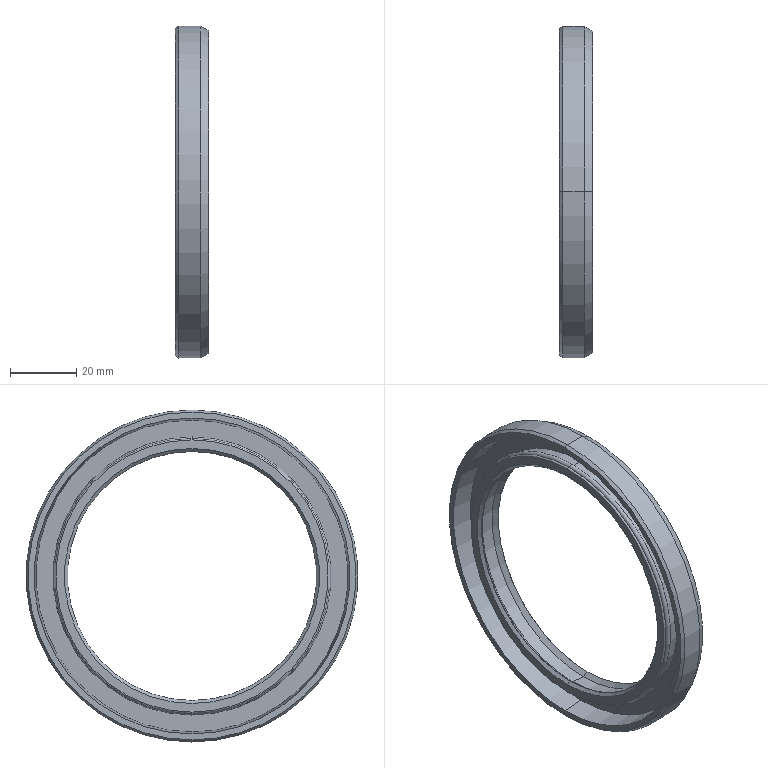Part | SolidWorks | features BaseBody 1 | 1 solid | 38 faces | box 10 x 100 x 100 mm | volume 19515 mm3 | cone 20 | torus 8 | cylinder 6 | plane 4 | commonest cylinder face diameters 78.465 x2 82.143 x2 100 x2
STEP:
#1=CARTESIAN_POINT('',(105.942,0.00006065,-37.5));
#2=VERTEX_POINT('',#1);
#3=CARTESIAN_POINT('',(105.871,0.0000607,-37.529));
#4=VERTEX_POINT('',#3);
#5=CARTESIAN_POINT('',(105.942,0.00006082,-37.6));
#6=DIRECTION('',(0.,-1.,-0.000001617));
#7=DIRECTION('',(0.,0.000001617,-1.));
#8=AXIS2_PLACEMENT_3D('',#5,#6,#7);
#9=CIRCLE('',#8,0.1);
#10=EDGE_CURVE('',#2,#4,#9,.T.);
#11=ORIENTED_EDGE('',*,*,#10,.F.);
#12=CARTESIAN_POINT('',(105.942,-0.00006065,37.5));
#13=VERTEX_POINT('',#12);
#14=CARTESIAN_POINT('',(105.942,0.,0.));
#15=DIRECTION('',(1.,0.,0.));
#16=DIRECTION('',(0.,1.,0.));
#17=AXIS2_PLACEMENT_3D('',#14,#15,#16);
#18=CIRCLE('',#17,37.5);
#19=EDGE_CURVE('',#2,#13,#18,.T.);
#20=ORIENTED_EDGE('',*,*,#19,.T.);
#21=CARTESIAN_POINT('',(105.871,-0.0000607,37.529));
#22=VERTEX_POINT('',#21);
#23=CARTESIAN_POINT('',(105.942,-0.00006082,37.6));
#24=DIRECTION('',(0.,1.,0.000001617));
#25=DIRECTION('',(0.,-0.000001617,1.));
#26=AXIS2_PLACEMENT_3D('',#23,#24,#25);
#27=CIRCLE('',#26,0.1);
#28=EDGE_CURVE('',#13,#22,#27,.T.);
#29=ORIENTED_EDGE('',*,*,#28,.T.);
#30=CARTESIAN_POINT('',(105.871,0.,37.529));
#31=VERTEX_POINT('',#30);
#32=CARTESIAN_POINT('',(105.871,0.,0.));
#33=DIRECTION('',(-1.,0.,0.));
#34=DIRECTION('',(0.,0.,-1.));
#35=AXIS2_PLACEMENT_3D('',#32,#33,#34);
#36=CIRCLE('',#35,37.529);
#37=EDGE_CURVE('',#22,#31,#36,.T.);
#38=ORIENTED_EDGE('',*,*,#37,.T.);
#39=CARTESIAN_POINT('',(105.871,0.,0.));
#40=DIRECTION('',(-1.,0.,0.));
#41=DIRECTION('',(0.,0.,-1.));
#42=AXIS2_PLACEMENT_3D('',#39,#40,#41);
#43=CIRCLE('',#42,37.529);
#44=EDGE_CURVE('',#31,#4,#43,.T.);
#45=ORIENTED_EDGE('',*,*,#44,.T.);
#46=EDGE_LOOP('',(#11,#20,#29,#38,#45));
#47=FACE_OUTER_BOUND('',#46,.T.);
#48=CARTESIAN_POINT('',(105.942,0.,0.));
#49=DIRECTION('',(1.,0.,0.));
#50=DIRECTION('',(0.,-0.000001617,1.));
#51=AXIS2_PLACEMENT_3D('',#48,#49,#50);
#52=TOROIDAL_SURFACE('',#51,37.6,0.1);
#53=ADVANCED_FACE('',(#47),#52,.T.);
#54=ORIENTED_EDGE('',*,*,#28,.F.);
#55=CARTESIAN_POINT('',(105.942,0.,0.));
#56=DIRECTION('',(1.,0.,0.));
#57=DIRECTION('',(0.,1.,0.));
#58=AXIS2_PLACEMENT_3D('',#55,#56,#57);
#59=CIRCLE('',#58,37.5);
#60=EDGE_CURVE('',#13,#2,#59,.T.);
#61=ORIENTED_EDGE('',*,*,#60,.T.);
#62=ORIENTED_EDGE('',*,*,#10,.T.);
#63=CARTESIAN_POINT('',(105.871,0.,-37.529));
#64=VERTEX_POINT('',#63);
#65=CARTESIAN_POINT('',(105.871,0.,0.));
#66=DIRECTION('',(-1.,0.,0.));
#67=DIRECTION('',(0.,0.,-1.));
#68=AXIS2_PLACEMENT_3D('',#65,#66,#67);
#69=CIRCLE('',#68,37.529);
#70=EDGE_CURVE('',#4,#64,#69,.T.);
#71=ORIENTED_EDGE('',*,*,#70,.T.);
#72=CARTESIAN_POINT('',(105.871,0.,0.));
#73=DIRECTION('',(-1.,0.,0.));
#74=DIRECTION('',(0.,0.,-1.));
#75=AXIS2_PLACEMENT_3D('',#72,#73,#74);
#76=CIRCLE('',#75,37.529);
#77=EDGE_CURVE('',#64,#22,#76,.T.);
#78=ORIENTED_EDGE('',*,*,#77,.T.);
#79=EDGE_LOOP('',(#54,#61,#62,#71,#78));
#80=FACE_OUTER_BOUND('',#79,.T.);
#81=CARTESIAN_POINT('',(105.942,0.,0.));
#82=DIRECTION('',(1.,0.,0.));
#83=DIRECTION('',(0.,-0.000001617,1.));
#84=AXIS2_PLACEMENT_3D('',#81,#82,#83);
#85=TOROIDAL_SURFACE('',#84,37.6,0.1);
#86=ADVANCED_FACE('',(#80),#85,.T.);
#87=ORIENTED_EDGE('',*,*,#60,.F.);
#88=CARTESIAN_POINT('',(106.002,-0.00006069,37.52));
#89=VERTEX_POINT('',#88);
#90=CARTESIAN_POINT('',(105.942,-0.00006082,37.6));
#91=DIRECTION('',(0.,1.,0.000001617));
#92=DIRECTION('',(0.,-0.000001617,1.));
#93=AXIS2_PLACEMENT_3D('',#90,#91,#92);
#94=CIRCLE('',#93,0.1);
#95=EDGE_CURVE('',#89,#13,#94,.T.);
#96=ORIENTED_EDGE('',*,*,#95,.F.);
#97=CARTESIAN_POINT('',(106.002,0.,-37.52));
#98=VERTEX_POINT('',#97);
#99=CARTESIAN_POINT('',(106.002,0.,0.));
#100=DIRECTION('',(-1.,0.,0.));
#101=DIRECTION('',(0.,0.,-1.));
#102=AXIS2_PLACEMENT_3D('',#99,#100,#101);
#103=CIRCLE('',#102,37.52);
#104=EDGE_CURVE('',#98,#89,#103,.T.);
#105=ORIENTED_EDGE('',*,*,#104,.F.);
#106=CARTESIAN_POINT('',(106.002,0.00006069,-37.52));
#107=VERTEX_POINT('',#106);
#108=CARTESIAN_POINT('',(106.002,0.,0.));
#109=DIRECTION('',(-1.,0.,0.));
#110=DIRECTION('',(0.,0.,-1.));
#111=AXIS2_PLACEMENT_3D('',#108,#109,#110);
#112=CIRCLE('',#111,37.52);
#113=EDGE_CURVE('',#107,#98,#112,.T.);
#114=ORIENTED_EDGE('',*,*,#113,.F.);
#115=CARTESIAN_POINT('',(105.942,0.00006082,-37.6));
#116=DIRECTION('',(0.,-1.,-0.000001617));
#117=DIRECTION('',(0.,0.000001617,-1.));
#118=AXIS2_PLACEMENT_3D('',#115,#116,#117);
#119=CIRCLE('',#118,0.1);
#120=EDGE_CURVE('',#107,#2,#119,.T.);
#121=ORIENTED_EDGE('',*,*,#120,.T.);
#122=EDGE_LOOP('',(#87,#96,#105,#114,#121));
#123=FACE_OUTER_BOUND('',#122,.T.);
#124=CARTESIAN_POINT('',(105.942,0.,0.));
#125=DIRECTION('',(1.,0.,0.));
#126=DIRECTION('',(0.,-0.000001617,1.));
#127=AXIS2_PLACEMENT_3D('',#124,#125,#126);
#128=TOROIDAL_SURFACE('',#127,37.6,0.1);
#129=ADVANCED_FACE('',(#123),#128,.T.);
#130=ORIENTED_EDGE('',*,*,#77,.F.);
#131=CARTESIAN_POINT('',(105.,0.,-38.4));
#132=VERTEX_POINT('',#131);
#133=CARTESIAN_POINT('',(142.4,0.,-1.));
#134=DIRECTION('',(-0.7071,0.,-0.7071));
#135=VECTOR('',#134,1000.);
#136=LINE('',#133,#135);
#137=EDGE_CURVE('',#64,#132,#136,.T.);
#138=ORIENTED_EDGE('',*,*,#137,.T.);
#139=CARTESIAN_POINT('',(105.,0.,38.4));
#140=VERTEX_POINT('',#139);
#141=CARTESIAN_POINT('',(105.,0.,0.));
#142=DIRECTION('',(-1.,0.,0.));
#143=DIRECTION('',(0.,0.,1.));
#144=AXIS2_PLACEMENT_3D('',#141,#142,#143);
#145=CIRCLE('',#144,38.4);
#146=EDGE_CURVE('',#132,#140,#145,.T.);
#147=ORIENTED_EDGE('',*,*,#146,.T.);
#148=CARTESIAN_POINT('',(142.4,0.,1.));
#149=DIRECTION('',(-0.7071,0.,0.7071));
#150=VECTOR('',#149,1000.);
#151=LINE('',#148,#150);
#152=EDGE_CURVE('',#31,#140,#151,.T.);
#153=ORIENTED_EDGE('',*,*,#152,.F.);
#154=ORIENTED_EDGE('',*,*,#37,.F.);
#155=EDGE_LOOP('',(#130,#138,#147,#153,#154));
#156=FACE_OUTER_BOUND('',#155,.T.);
#157=CARTESIAN_POINT('',(142.4,0.,0.));
#158=DIRECTION('',(-1.,0.,0.));
#159=DIRECTION('',(0.,0.,1.));
#160=AXIS2_PLACEMENT_3D('',#157,#158,#159);
#161=CONICAL_SURFACE('',#160,1.,0.7854);
#162=ADVANCED_FACE('',(#156),#161,.F.);
#163=CARTESIAN_POINT('',(105.,-0.000000008,40.996));
#164=VERTEX_POINT('',#163);
#165=CARTESIAN_POINT('',(105.,0.,-40.996));
#166=VERTEX_POINT('',#165);
#167=CARTESIAN_POINT('',(105.,0.,0.));
#168=DIRECTION('',(-1.,0.,0.));
#169=DIRECTION('',(0.,0.,-1.));
#170=AXIS2_PLACEMENT_3D('',#167,#168,#169);
#171=CIRCLE('',#170,40.996);
#172=EDGE_CURVE('',#164,#166,#171,.T.);
#173=ORIENTED_EDGE('',*,*,#172,.F.);
#174=CARTESIAN_POINT('',(105.799,0.,41.021));
#175=VERTEX_POINT('',#174);
#176=CARTESIAN_POINT('',(105.4,-0.000000007,40.996));
#177=DIRECTION('',(0.,1.,0.));
#178=DIRECTION('',(0.,0.,1.));
#179=AXIS2_PLACEMENT_3D('',#176,#177,#178);
#180=CIRCLE('',#179,0.4);
#181=EDGE_CURVE('',#164,#175,#180,.T.);
#182=ORIENTED_EDGE('',*,*,#181,.T.);
#183=CARTESIAN_POINT('',(105.799,0.000000027,-41.021));
#184=VERTEX_POINT('',#183);
#185=CARTESIAN_POINT('',(105.799,0.,0.));
#186=DIRECTION('',(-1.,0.,0.));
#187=DIRECTION('',(0.,0.,1.));
#188=AXIS2_PLACEMENT_3D('',#185,#186,#187);
#189=CIRCLE('',#188,41.021);
#190=EDGE_CURVE('',#175,#184,#189,.T.);
#191=ORIENTED_EDGE('',*,*,#190,.T.);
#192=CARTESIAN_POINT('',(105.4,0.000000007,-40.996));
#193=DIRECTION('',(0.,-1.,0.));
#194=DIRECTION('',(0.,0.,-1.));
#195=AXIS2_PLACEMENT_3D('',#192,#193,#194);
#196=CIRCLE('',#195,0.4);
#197=EDGE_CURVE('',#166,#184,#196,.T.);
#198=ORIENTED_EDGE('',*,*,#197,.F.);
#199=EDGE_LOOP('',(#173,#182,#191,#198));
#200=FACE_OUTER_BOUND('',#199,.T.);
#201=CARTESIAN_POINT('',(105.4,0.,0.));
#202=DIRECTION('',(1.,0.,0.));
#203=DIRECTION('',(0.,0.,-1.));
#204=AXIS2_PLACEMENT_3D('',#201,#202,#203);
#205=TOROIDAL_SURFACE('',#204,40.996,0.4);
#206=ADVANCED_FACE('',(#200),#205,.T.);
#207=CARTESIAN_POINT('',(105.799,0.,0.));
#208=DIRECTION('',(-1.,0.,0.));
#209=DIRECTION('',(0.,0.,1.));
#210=AXIS2_PLACEMENT_3D('',#207,#208,#209);
#211=CIRCLE('',#210,41.021);
#212=EDGE_CURVE('',#184,#175,#211,.T.);
#213=ORIENTED_EDGE('',*,*,#212,.F.);
#214=CARTESIAN_POINT('',(107.398,0.,-41.071));
#215=VERTEX_POINT('',#214);
#216=CARTESIAN_POINT('',(106.598,0.000000027,-41.071));
#217=DIRECTION('',(0.,-1.,-0.000000001));
#218=DIRECTION('',(0.,0.000000001,-1.));
#219=AXIS2_PLACEMENT_3D('',#216,#217,#218);
#220=CIRCLE('',#219,0.8);
#221=EDGE_CURVE('',#184,#215,#220,.T.);
#222=ORIENTED_EDGE('',*,*,#221,.T.);
#223=CARTESIAN_POINT('',(107.398,0.,41.071));
#224=VERTEX_POINT('',#223);
#225=CARTESIAN_POINT('',(107.398,0.,0.));
#226=DIRECTION('',(-1.,0.,0.));
#227=DIRECTION('',(0.,0.,-1.));
#228=AXIS2_PLACEMENT_3D('',#225,#226,#227);
#229=CIRCLE('',#228,41.071);
#230=EDGE_CURVE('',#215,#224,#229,.T.);
#231=ORIENTED_EDGE('',*,*,#230,.T.);
#232=CARTESIAN_POINT('',(106.598,-0.000000027,41.071));
#233=DIRECTION('',(0.,1.,0.000000001));
#234=DIRECTION('',(0.,-0.000000001,1.));
#235=AXIS2_PLACEMENT_3D('',#232,#233,#234);
#236=CIRCLE('',#235,0.8);
#237=EDGE_CURVE('',#175,#224,#236,.T.);
#238=ORIENTED_EDGE('',*,*,#237,.F.);
#239=EDGE_LOOP('',(#213,#222,#231,#238));
#240=FACE_OUTER_BOUND('',#239,.T.);
#241=CARTESIAN_POINT('',(106.598,0.,0.));
#242=DIRECTION('',(1.,0.,0.));
#243=DIRECTION('',(0.,-0.000000001,1.));
#244=AXIS2_PLACEMENT_3D('',#241,#242,#243);
#245=TOROIDAL_SURFACE('',#244,41.071,0.8);
#246=ADVANCED_FACE('',(#240),#245,.T.);
#247=CARTESIAN_POINT('',(107.398,0.,0.));
#248=DIRECTION('',(-1.,0.,0.));
#249=DIRECTION('',(0.,0.,-1.));
#250=AXIS2_PLACEMENT_3D('',#247,#248,#249);
#251=CIRCLE('',#250,41.071);
#252=EDGE_CURVE('',#224,#215,#251,.T.);
#253=ORIENTED_EDGE('',*,*,#252,.F.);
#254=CARTESIAN_POINT('',(110.667,0.,41.071));
#255=VERTEX_POINT('',#254);
#256=CARTESIAN_POINT('',(107.398,0.,41.071));
#257=DIRECTION('',(1.,0.,0.));
#258=VECTOR('',#257,1000.);
#259=LINE('',#256,#258);
#260=EDGE_CURVE('',#224,#255,#259,.T.);
#261=ORIENTED_EDGE('',*,*,#260,.T.);
#262=CARTESIAN_POINT('',(110.667,0.,-41.071));
#263=VERTEX_POINT('',#262);
#264=CARTESIAN_POINT('',(110.667,0.,0.));
#265=DIRECTION('',(-1.,0.,0.));
#266=DIRECTION('',(0.,0.,1.));
#267=AXIS2_PLACEMENT_3D('',#264,#265,#266);
#268=CIRCLE('',#267,41.071);
#269=EDGE_CURVE('',#255,#263,#268,.T.);
#270=ORIENTED_EDGE('',*,*,#269,.T.);
#271=CARTESIAN_POINT('',(107.398,0.,-41.071));
#272=DIRECTION('',(1.,0.,0.));
#273=VECTOR('',#272,1000.);
#274=LINE('',#271,#273);
#275=EDGE_CURVE('',#215,#263,#274,.T.);
#276=ORIENTED_EDGE('',*,*,#275,.F.);
#277=EDGE_LOOP('',(#253,#261,#270,#276));
#278=FACE_OUTER_BOUND('',#277,.T.);
#279=CARTESIAN_POINT('',(107.398,0.,0.));
#280=DIRECTION('',(1.,0.,0.));
#281=DIRECTION('',(0.,0.,-1.));
#282=AXIS2_PLACEMENT_3D('',#279,#280,#281);
#283=CYLINDRICAL_SURFACE('',#282,41.071);
#284=ADVANCED_FACE('',(#278),#283,.T.);
#285=CARTESIAN_POINT('',(110.667,0.,-46.982));
#286=VERTEX_POINT('',#285);
#287=CARTESIAN_POINT('',(110.667,0.,46.982));
#288=VERTEX_POINT('',#287);
#289=CARTESIAN_POINT('',(110.667,0.,0.));
#290=DIRECTION('',(-1.,0.,0.));
#291=DIRECTION('',(0.,0.,1.));
#292=AXIS2_PLACEMENT_3D('',#289,#290,#291);
#293=CIRCLE('',#292,46.982);
#294=EDGE_CURVE('',#286,#288,#293,.T.);
#295=ORIENTED_EDGE('',*,*,#294,.F.);
#296=CARTESIAN_POINT('',(104.,0.,-47.565));
#297=VERTEX_POINT('',#296);
#298=CARTESIAN_POINT('',(476.751,0.,-14.953));
#299=DIRECTION('',(-0.9962,0.,-0.08716));
#300=VECTOR('',#299,1000.);
#301=LINE('',#298,#300);
#302=EDGE_CURVE('',#286,#297,#301,.T.);
#303=ORIENTED_EDGE('',*,*,#302,.T.);
#304=CARTESIAN_POINT('',(104.,0.,47.565));
#305=VERTEX_POINT('',#304);
#306=CARTESIAN_POINT('',(104.,0.,0.));
#307=DIRECTION('',(-1.,0.,0.));
#308=DIRECTION('',(0.,0.,-1.));
#309=AXIS2_PLACEMENT_3D('',#306,#307,#308);
#310=CIRCLE('',#309,47.565);
#311=EDGE_CURVE('',#297,#305,#310,.T.);
#312=ORIENTED_EDGE('',*,*,#311,.T.);
#313=CARTESIAN_POINT('',(476.751,0.,14.953));
#314=DIRECTION('',(-0.9962,0.,0.08716));
#315=VECTOR('',#314,1000.);
#316=LINE('',#313,#315);
#317=EDGE_CURVE('',#288,#305,#316,.T.);
#318=ORIENTED_EDGE('',*,*,#317,.F.);
#319=EDGE_LOOP('',(#295,#303,#312,#318));
#320=FACE_OUTER_BOUND('',#319,.T.);
#321=CARTESIAN_POINT('',(476.751,0.,0.));
#322=DIRECTION('',(-1.,0.,0.));
#323=DIRECTION('',(0.,0.,1.));
#324=AXIS2_PLACEMENT_3D('',#321,#322,#323);
#325=CONICAL_SURFACE('',#324,14.953,0.08727);
#326=ADVANCED_FACE('',(#320),#325,.F.);
#327=CARTESIAN_POINT('',(104.,0.,49.351));
#328=VERTEX_POINT('',#327);
#329=CARTESIAN_POINT('',(104.,0.,-49.351));
#330=VERTEX_POINT('',#329);
#331=CARTESIAN_POINT('',(104.,0.,0.));
#332=DIRECTION('',(-1.,0.,0.));
#333=DIRECTION('',(0.,0.,-1.));
#334=AXIS2_PLACEMENT_3D('',#331,#332,#333);
#335=CIRCLE('',#334,49.351);
#336=EDGE_CURVE('',#328,#330,#335,.T.);
#337=ORIENTED_EDGE('',*,*,#336,.F.);
#338=CARTESIAN_POINT('',(105.,0.,50.));
#339=VERTEX_POINT('',#338);
#340=CARTESIAN_POINT('',(29.007,0.,0.6494));
#341=DIRECTION('',(0.8387,0.,0.5446));
#342=VECTOR('',#341,1000.);
#343=LINE('',#340,#342);
#344=EDGE_CURVE('',#328,#339,#343,.T.);
#345=ORIENTED_EDGE('',*,*,#344,.T.);
#346=CARTESIAN_POINT('',(105.,0.,-50.));
#347=VERTEX_POINT('',#346);
#348=CARTESIAN_POINT('',(105.,0.,0.));
#349=DIRECTION('',(-1.,0.,0.));
#350=DIRECTION('',(0.,0.,1.));
#351=AXIS2_PLACEMENT_3D('',#348,#349,#350);
#352=CIRCLE('',#351,50.);
#353=EDGE_CURVE('',#339,#347,#352,.T.);
#354=ORIENTED_EDGE('',*,*,#353,.T.);
#355=CARTESIAN_POINT('',(29.007,0.,-0.6494));
#356=DIRECTION('',(0.8387,0.,-0.5446));
#357=VECTOR('',#356,1000.);
#358=LINE('',#355,#357);
#359=EDGE_CURVE('',#330,#347,#358,.T.);
#360=ORIENTED_EDGE('',*,*,#359,.F.);
#361=EDGE_LOOP('',(#337,#345,#354,#360));
#362=FACE_OUTER_BOUND('',#361,.T.);
#363=CARTESIAN_POINT('',(29.007,0.,0.));
#364=DIRECTION('',(1.,0.,0.));
#365=DIRECTION('',(0.,0.,-1.));
#366=AXIS2_PLACEMENT_3D('',#363,#364,#365);
#367=CONICAL_SURFACE('',#366,0.6494,0.576);
#368=ADVANCED_FACE('',(#362),#367,.T.);
#369=CARTESIAN_POINT('',(105.,0.,0.));
#370=DIRECTION('',(-1.,0.,0.));
#371=DIRECTION('',(0.,0.,1.));
#372=AXIS2_PLACEMENT_3D('',#369,#370,#371);
#373=CIRCLE('',#372,50.);
#374=EDGE_CURVE('',#347,#339,#373,.T.);
#375=ORIENTED_EDGE('',*,*,#374,.F.);
#376=CARTESIAN_POINT('',(111.5,0.,-50.));
#377=VERTEX_POINT('',#376);
#378=CARTESIAN_POINT('',(105.,0.,-50.));
#379=DIRECTION('',(1.,0.,0.));
#380=VECTOR('',#379,1000.);
#381=LINE('',#378,#380);
#382=EDGE_CURVE('',#347,#377,#381,.T.);
#383=ORIENTED_EDGE('',*,*,#382,.T.);
#384=CARTESIAN_POINT('',(111.5,0.,50.));
#385=VERTEX_POINT('',#384);
#386=CARTESIAN_POINT('',(111.5,0.,0.));
#387=DIRECTION('',(-1.,0.,0.));
#388=DIRECTION('',(0.,0.,-1.));
#389=AXIS2_PLACEMENT_3D('',#386,#387,#388);
#390=CIRCLE('',#389,50.);
#391=EDGE_CURVE('',#377,#385,#390,.T.);
#392=ORIENTED_EDGE('',*,*,#391,.T.);
#393=CARTESIAN_POINT('',(105.,0.,50.));
#394=DIRECTION('',(1.,0.,0.));
#395=VECTOR('',#394,1000.);
#396=LINE('',#393,#395);
#397=EDGE_CURVE('',#339,#385,#396,.T.);
#398=ORIENTED_EDGE('',*,*,#397,.F.);
#399=EDGE_LOOP('',(#375,#383,#392,#398));
#400=FACE_OUTER_BOUND('',#399,.T.);
#401=CARTESIAN_POINT('',(105.,0.,0.));
#402=DIRECTION('',(1.,0.,0.));
#403=DIRECTION('',(0.,0.,1.));
#404=AXIS2_PLACEMENT_3D('',#401,#402,#403);
#405=CYLINDRICAL_SURFACE('',#404,50.);
#406=ADVANCED_FACE('',(#400),#405,.T.);
#407=CARTESIAN_POINT('',(114.,0.,48.557));
#408=VERTEX_POINT('',#407);
#409=CARTESIAN_POINT('',(114.,0.,-48.557));
#410=VERTEX_POINT('',#409);
#411=CARTESIAN_POINT('',(114.,0.,0.));
#412=DIRECTION('',(-1.,0.,0.));
#413=DIRECTION('',(0.,0.,1.));
#414=AXIS2_PLACEMENT_3D('',#411,#412,#413);
#415=CIRCLE('',#414,48.557);
#416=EDGE_CURVE('',#408,#410,#415,.T.);
#417=ORIENTED_EDGE('',*,*,#416,.T.);
#418=CARTESIAN_POINT('',(197.103,0.,-0.5774));
#419=DIRECTION('',(-0.866,0.,-0.5));
#420=VECTOR('',#419,1000.);
#421=LINE('',#418,#420);
#422=EDGE_CURVE('',#410,#377,#421,.T.);
#423=ORIENTED_EDGE('',*,*,#422,.T.);
#424=CARTESIAN_POINT('',(111.5,0.,0.));
#425=DIRECTION('',(-1.,0.,0.));
#426=DIRECTION('',(0.,0.,-1.));
#427=AXIS2_PLACEMENT_3D('',#424,#425,#426);
#428=CIRCLE('',#427,50.);
#429=EDGE_CURVE('',#385,#377,#428,.T.);
#430=ORIENTED_EDGE('',*,*,#429,.F.);
#431=CARTESIAN_POINT('',(197.103,0.,0.5774));
#432=DIRECTION('',(-0.866,0.,0.5));
#433=VECTOR('',#432,1000.);
#434=LINE('',#431,#433);
#435=EDGE_CURVE('',#408,#385,#434,.T.);
#436=ORIENTED_EDGE('',*,*,#435,.F.);
#437=EDGE_LOOP('',(#417,#423,#430,#436));
#438=FACE_OUTER_BOUND('',#437,.T.);
#439=CARTESIAN_POINT('',(197.103,0.,0.));
#440=DIRECTION('',(-1.,0.,0.));
#441=DIRECTION('',(0.,0.,1.));
#442=AXIS2_PLACEMENT_3D('',#439,#440,#441);
#443=CONICAL_SURFACE('',#442,0.5774,0.5236);
#444=ADVANCED_FACE('',(#438),#443,.T.);
#445=CARTESIAN_POINT('',(112.583,0.,39.232));
#446=VERTEX_POINT('',#445);
#447=CARTESIAN_POINT('',(112.583,0.,-39.232));
#448=VERTEX_POINT('',#447);
#449=CARTESIAN_POINT('',(112.583,0.,0.));
#450=DIRECTION('',(-1.,0.,0.));
#451=DIRECTION('',(0.,0.,1.));
#452=AXIS2_PLACEMENT_3D('',#449,#450,#451);
#453=CIRCLE('',#452,39.232);
#454=EDGE_CURVE('',#446,#448,#453,.T.);
#455=ORIENTED_EDGE('',*,*,#454,.T.);
#456=CARTESIAN_POINT('',(114.,0.,-39.232));
#457=VERTEX_POINT('',#456);
#458=CARTESIAN_POINT('',(112.583,0.,-39.232));
#459=DIRECTION('',(1.,0.,0.));
#460=VECTOR('',#459,1000.);
#461=LINE('',#458,#460);
#462=EDGE_CURVE('',#448,#457,#461,.T.);
#463=ORIENTED_EDGE('',*,*,#462,.T.);
#464=CARTESIAN_POINT('',(114.,0.,39.232));
#465=VERTEX_POINT('',#464);
#466=CARTESIAN_POINT('',(114.,0.,0.));
#467=DIRECTION('',(-1.,0.,0.));
#468=DIRECTION('',(0.,0.,-1.));
#469=AXIS2_PLACEMENT_3D('',#466,#467,#468);
#470=CIRCLE('',#469,39.232);
#471=EDGE_CURVE('',#465,#457,#470,.T.);
#472=ORIENTED_EDGE('',*,*,#471,.F.);
#473=CARTESIAN_POINT('',(112.583,0.,39.232));
#474=DIRECTION('',(1.,0.,0.));
#475=VECTOR('',#474,1000.);
#476=LINE('',#473,#475);
#477=EDGE_CURVE('',#446,#465,#476,.T.);
#478=ORIENTED_EDGE('',*,*,#477,.F.);
#479=EDGE_LOOP('',(#455,#463,#472,#478));
#480=FACE_OUTER_BOUND('',#479,.T.);
#481=CARTESIAN_POINT('',(112.583,0.,0.));
#482=DIRECTION('',(1.,0.,0.));
#483=DIRECTION('',(0.,0.,1.));
#484=AXIS2_PLACEMENT_3D('',#481,#482,#483);
#485=CYLINDRICAL_SURFACE('',#484,39.232);
#486=ADVANCED_FACE('',(#480),#485,.F.);
#487=CARTESIAN_POINT('',(113.714,0.,38.349));
#488=VERTEX_POINT('',#487);
#489=CARTESIAN_POINT('',(113.714,0.,-38.349));
#490=VERTEX_POINT('',#489);
#491=CARTESIAN_POINT('',(113.714,0.,0.));
#492=DIRECTION('',(-1.,0.,0.));
#493=DIRECTION('',(0.,0.,-1.));
#494=AXIS2_PLACEMENT_3D('',#491,#492,#493);
#495=CIRCLE('',#494,38.349);
#496=EDGE_CURVE('',#488,#490,#495,.T.);
#497=ORIENTED_EDGE('',*,*,#496,.T.);
#498=CARTESIAN_POINT('',(161.798,0.,-0.7813));
#499=DIRECTION('',(-0.788,0.,-0.6157));
#500=VECTOR('',#499,1000.);
#501=LINE('',#498,#500);
#502=EDGE_CURVE('',#490,#448,#501,.T.);
#503=ORIENTED_EDGE('',*,*,#502,.T.);
#504=ORIENTED_EDGE('',*,*,#454,.F.);
#505=CARTESIAN_POINT('',(161.798,0.,0.7813));
#506=DIRECTION('',(-0.788,0.,0.6157));
#507=VECTOR('',#506,1000.);
#508=LINE('',#505,#507);
#509=EDGE_CURVE('',#488,#446,#508,.T.);
#510=ORIENTED_EDGE('',*,*,#509,.F.);
#511=EDGE_LOOP('',(#497,#503,#504,#510));
#512=FACE_OUTER_BOUND('',#511,.T.);
#513=CARTESIAN_POINT('',(161.798,0.,0.));
#514=DIRECTION('',(-1.,0.,0.));
#515=DIRECTION('',(0.,0.,1.));
#516=AXIS2_PLACEMENT_3D('',#513,#514,#515);
#517=CONICAL_SURFACE('',#516,0.7813,0.6632);
#518=ADVANCED_FACE('',(#512),#517,.T.);
#519=CARTESIAN_POINT('',(113.275,0.,-37.786));
#520=VERTEX_POINT('',#519);
#521=CARTESIAN_POINT('',(113.275,0.,37.786));
#522=VERTEX_POINT('',#521);
#523=CARTESIAN_POINT('',(113.275,0.,0.));
#524=DIRECTION('',(-1.,0.,0.));
#525=DIRECTION('',(0.,0.,1.));
#526=AXIS2_PLACEMENT_3D('',#523,#524,#525);
#527=CIRCLE('',#526,37.786);
#528=EDGE_CURVE('',#520,#522,#527,.T.);
#529=ORIENTED_EDGE('',*,*,#528,.T.);
#530=CARTESIAN_POINT('',(84.753,0.,1.28));
#531=DIRECTION('',(0.6157,0.,0.788));
#532=VECTOR('',#531,1000.);
#533=LINE('',#530,#532);
#534=EDGE_CURVE('',#522,#488,#533,.T.);
#535=ORIENTED_EDGE('',*,*,#534,.T.);
#536=CARTESIAN_POINT('',(113.714,0.,0.));
#537=DIRECTION('',(-1.,0.,0.));
#538=DIRECTION('',(0.,0.,-1.));
#539=AXIS2_PLACEMENT_3D('',#536,#537,#538);
#540=CIRCLE('',#539,38.349);
#541=EDGE_CURVE('',#490,#488,#540,.T.);
#542=ORIENTED_EDGE('',*,*,#541,.F.);
#543=CARTESIAN_POINT('',(84.753,0.,-1.28));
#544=DIRECTION('',(0.6157,0.,-0.788));
#545=VECTOR('',#544,1000.);
#546=LINE('',#543,#545);
#547=EDGE_CURVE('',#520,#490,#546,.T.);
#548=ORIENTED_EDGE('',*,*,#547,.F.);
#549=EDGE_LOOP('',(#529,#535,#542,#548));
#550=FACE_OUTER_BOUND('',#549,.T.);
#551=CARTESIAN_POINT('',(84.753,0.,0.));
#552=DIRECTION('',(1.,0.,0.));
#553=DIRECTION('',(0.,0.,-1.));
#554=AXIS2_PLACEMENT_3D('',#551,#552,#553);
#555=CONICAL_SURFACE('',#554,1.28,0.9076);
#556=ADVANCED_FACE('',(#550),#555,.F.);
#557=ORIENTED_EDGE('',*,*,#528,.F.);
#558=CARTESIAN_POINT('',(111.773,0.,-38.959));
#559=VERTEX_POINT('',#558);
#560=CARTESIAN_POINT('',(160.638,0.,-0.7813));
#561=DIRECTION('',(-0.788,0.,-0.6157));
#562=VECTOR('',#561,1000.);
#563=LINE('',#560,#562);
#564=EDGE_CURVE('',#520,#559,#563,.T.);
#565=ORIENTED_EDGE('',*,*,#564,.T.);
#566=CARTESIAN_POINT('',(111.773,0.,38.959));
#567=VERTEX_POINT('',#566);
#568=CARTESIAN_POINT('',(111.773,0.,0.));
#569=DIRECTION('',(-1.,0.,0.));
#570=DIRECTION('',(0.,0.,-1.));
#571=AXIS2_PLACEMENT_3D('',#568,#569,#570);
#572=CIRCLE('',#571,38.959);
#573=EDGE_CURVE('',#559,#567,#572,.T.);
#574=ORIENTED_EDGE('',*,*,#573,.T.);
#575=CARTESIAN_POINT('',(160.638,0.,0.7813));
#576=DIRECTION('',(-0.788,0.,0.6157));
#577=VECTOR('',#576,1000.);
#578=LINE('',#575,#577);
#579=EDGE_CURVE('',#522,#567,#578,.T.);
#580=ORIENTED_EDGE('',*,*,#579,.F.);
#581=EDGE_LOOP('',(#557,#565,#574,#580));
#582=FACE_OUTER_BOUND('',#581,.T.);
#583=CARTESIAN_POINT('',(160.638,0.,0.));
#584=DIRECTION('',(-1.,0.,0.));
#585=DIRECTION('',(0.,0.,1.));
#586=AXIS2_PLACEMENT_3D('',#583,#584,#585);
#587=CONICAL_SURFACE('',#586,0.7813,0.6632);
#588=ADVANCED_FACE('',(#582),#587,.F.);
#589=CARTESIAN_POINT('',(106.977,0.,-38.37));
#590=VERTEX_POINT('',#589);
#591=CARTESIAN_POINT('',(106.977,0.,38.37));
#592=VERTEX_POINT('',#591);
#593=CARTESIAN_POINT('',(106.977,0.,0.));
#594=DIRECTION('',(-1.,0.,0.));
#595=DIRECTION('',(0.,0.,1.));
#596=AXIS2_PLACEMENT_3D('',#593,#594,#595);
#597=CIRCLE('',#596,38.37);
#598=EDGE_CURVE('',#590,#592,#597,.T.);
#599=ORIENTED_EDGE('',*,*,#598,.T.);
#600=CARTESIAN_POINT('',(-193.087,0.,1.527));
#601=DIRECTION('',(0.9925,0.,0.1219));
#602=VECTOR('',#601,1000.);
#603=LINE('',#600,#602);
#604=EDGE_CURVE('',#592,#567,#603,.T.);
#605=ORIENTED_EDGE('',*,*,#604,.T.);
#606=ORIENTED_EDGE('',*,*,#573,.F.);
#607=CARTESIAN_POINT('',(-193.087,0.,-1.527));
#608=DIRECTION('',(0.9925,0.,-0.1219));
#609=VECTOR('',#608,1000.);
#610=LINE('',#607,#609);
#611=EDGE_CURVE('',#590,#559,#610,.T.);
#612=ORIENTED_EDGE('',*,*,#611,.F.);
#613=EDGE_LOOP('',(#599,#605,#606,#612));
#614=FACE_OUTER_BOUND('',#613,.T.);
#615=CARTESIAN_POINT('',(-193.087,0.,0.));
#616=DIRECTION('',(1.,0.,0.));
#617=DIRECTION('',(0.,0.,-1.));
#618=AXIS2_PLACEMENT_3D('',#615,#616,#617);
#619=CONICAL_SURFACE('',#618,1.527,0.1222);
#620=ADVANCED_FACE('',(#614),#619,.F.);
#621=CARTESIAN_POINT('',(106.904,0.,-38.2));
#622=VERTEX_POINT('',#621);
#623=CARTESIAN_POINT('',(106.904,0.,38.2));
#624=VERTEX_POINT('',#623);
#625=CARTESIAN_POINT('',(106.904,0.,0.));
#626=DIRECTION('',(-1.,0.,0.));
#627=DIRECTION('',(0.,0.,-1.));
#628=AXIS2_PLACEMENT_3D('',#625,#626,#627);
#629=CIRCLE('',#628,38.2);
#630=EDGE_CURVE('',#622,#624,#629,.T.);
#631=ORIENTED_EDGE('',*,*,#630,.T.);
#632=CARTESIAN_POINT('',(91.689,0.,2.356));
#633=DIRECTION('',(0.3907,0.,0.9205));
#634=VECTOR('',#633,1000.);
#635=LINE('',#632,#634);
#636=EDGE_CURVE('',#624,#592,#635,.T.);
#637=ORIENTED_EDGE('',*,*,#636,.T.);
#638=ORIENTED_EDGE('',*,*,#598,.F.);
#639=CARTESIAN_POINT('',(91.689,0.,-2.356));
#640=DIRECTION('',(0.3907,0.,-0.9205));
#641=VECTOR('',#640,1000.);
#642=LINE('',#639,#641);
#643=EDGE_CURVE('',#622,#590,#642,.T.);
#644=ORIENTED_EDGE('',*,*,#643,.F.);
#645=EDGE_LOOP('',(#631,#637,#638,#644));
#646=FACE_OUTER_BOUND('',#645,.T.);
#647=CARTESIAN_POINT('',(91.689,0.,0.));
#648=DIRECTION('',(1.,0.,0.));
#649=DIRECTION('',(0.,0.,-1.));
#650=AXIS2_PLACEMENT_3D('',#647,#648,#649);
#651=CONICAL_SURFACE('',#650,2.356,1.169);
#652=ADVANCED_FACE('',(#646),#651,.F.);
#653=ORIENTED_EDGE('',*,*,#104,.T.);
#654=CARTESIAN_POINT('',(106.002,0.,37.52));
#655=VERTEX_POINT('',#654);
#656=CARTESIAN_POINT('',(106.002,0.,0.));
#657=DIRECTION('',(-1.,0.,0.));
#658=DIRECTION('',(0.,0.,-1.));
#659=AXIS2_PLACEMENT_3D('',#656,#657,#658);
#660=CIRCLE('',#659,37.52);
#661=EDGE_CURVE('',#89,#655,#660,.T.);
#662=ORIENTED_EDGE('',*,*,#661,.T.);
#663=CARTESIAN_POINT('',(57.211,0.,0.7536));
#664=DIRECTION('',(0.7986,0.,0.6018));
#665=VECTOR('',#664,1000.);
#666=LINE('',#663,#665);
#667=EDGE_CURVE('',#655,#624,#666,.T.);
#668=ORIENTED_EDGE('',*,*,#667,.T.);
#669=ORIENTED_EDGE('',*,*,#630,.F.);
#670=CARTESIAN_POINT('',(57.211,0.,-0.7536));
#671=DIRECTION('',(0.7986,0.,-0.6018));
#672=VECTOR('',#671,1000.);
#673=LINE('',#670,#672);
#674=EDGE_CURVE('',#98,#622,#673,.T.);
#675=ORIENTED_EDGE('',*,*,#674,.F.);
#676=EDGE_LOOP('',(#653,#662,#668,#669,#675));
#677=FACE_OUTER_BOUND('',#676,.T.);
#678=CARTESIAN_POINT('',(57.211,0.,0.));
#679=DIRECTION('',(1.,0.,0.));
#680=DIRECTION('',(0.,0.,-1.));
#681=AXIS2_PLACEMENT_3D('',#678,#679,#680);
#682=CONICAL_SURFACE('',#681,0.7536,0.6458);
#683=ADVANCED_FACE('',(#677),#682,.F.);
#684=ORIENTED_EDGE('',*,*,#667,.F.);
#685=CARTESIAN_POINT('',(106.002,0.,0.));
#686=DIRECTION('',(-1.,0.,0.));
#687=DIRECTION('',(0.,0.,-1.));
#688=AXIS2_PLACEMENT_3D('',#685,#686,#687);
#689=CIRCLE('',#688,37.52);
#690=EDGE_CURVE('',#655,#107,#689,.T.);
#691=ORIENTED_EDGE('',*,*,#690,.T.);
#692=ORIENTED_EDGE('',*,*,#113,.T.);
#693=ORIENTED_EDGE('',*,*,#674,.T.);
#694=CARTESIAN_POINT('',(106.904,0.,0.));
#695=DIRECTION('',(-1.,0.,0.));
#696=DIRECTION('',(0.,0.,-1.));
#697=AXIS2_PLACEMENT_3D('',#694,#695,#696);
#698=CIRCLE('',#697,38.2);
#699=EDGE_CURVE('',#624,#622,#698,.T.);
#700=ORIENTED_EDGE('',*,*,#699,.F.);
#701=EDGE_LOOP('',(#684,#691,#692,#693,#700));
#702=FACE_OUTER_BOUND('',#701,.T.);
#703=CARTESIAN_POINT('',(57.211,0.,0.));
#704=DIRECTION('',(1.,0.,0.));
#705=DIRECTION('',(0.,0.,-1.));
#706=AXIS2_PLACEMENT_3D('',#703,#704,#705);
#707=CONICAL_SURFACE('',#706,0.7536,0.6458);
#708=ADVANCED_FACE('',(#702),#707,.F.);
#709=ORIENTED_EDGE('',*,*,#636,.F.);
#710=ORIENTED_EDGE('',*,*,#699,.T.);
#711=ORIENTED_EDGE('',*,*,#643,.T.);
#712=CARTESIAN_POINT('',(106.977,0.,0.));
#713=DIRECTION('',(-1.,0.,0.));
#714=DIRECTION('',(0.,0.,1.));
#715=AXIS2_PLACEMENT_3D('',#712,#713,#714);
#716=CIRCLE('',#715,38.37);
#717=EDGE_CURVE('',#592,#590,#716,.T.);
#718=ORIENTED_EDGE('',*,*,#717,.F.);
#719=EDGE_LOOP('',(#709,#710,#711,#718));
#720=FACE_OUTER_BOUND('',#719,.T.);
#721=CARTESIAN_POINT('',(91.689,0.,0.));
#722=DIRECTION('',(1.,0.,0.));
#723=DIRECTION('',(0.,0.,-1.));
#724=AXIS2_PLACEMENT_3D('',#721,#722,#723);
#725=CONICAL_SURFACE('',#724,2.356,1.169);
#726=ADVANCED_FACE('',(#720),#725,.F.);
#727=ORIENTED_EDGE('',*,*,#604,.F.);
#728=ORIENTED_EDGE('',*,*,#717,.T.);
#729=ORIENTED_EDGE('',*,*,#611,.T.);
#730=CARTESIAN_POINT('',(111.773,0.,0.));
#731=DIRECTION('',(-1.,0.,0.));
#732=DIRECTION('',(0.,0.,-1.));
#733=AXIS2_PLACEMENT_3D('',#730,#731,#732);
#734=CIRCLE('',#733,38.959);
#735=EDGE_CURVE('',#567,#559,#734,.T.);
#736=ORIENTED_EDGE('',*,*,#735,.F.);
#737=EDGE_LOOP('',(#727,#728,#729,#736));
#738=FACE_OUTER_BOUND('',#737,.T.);
#739=CARTESIAN_POINT('',(-193.087,0.,0.));
#740=DIRECTION('',(1.,0.,0.));
#741=DIRECTION('',(0.,0.,-1.));
#742=AXIS2_PLACEMENT_3D('',#739,#740,#741);
#743=CONICAL_SURFACE('',#742,1.527,0.1222);
#744=ADVANCED_FACE('',(#738),#743,.F.);
#745=ORIENTED_EDGE('',*,*,#564,.F.);
#746=CARTESIAN_POINT('',(113.275,0.,0.));
#747=DIRECTION('',(-1.,0.,0.));
#748=DIRECTION('',(0.,0.,1.));
#749=AXIS2_PLACEMENT_3D('',#746,#747,#748);
#750=CIRCLE('',#749,37.786);
#751=EDGE_CURVE('',#522,#520,#750,.T.);
#752=ORIENTED_EDGE('',*,*,#751,.F.);
#753=ORIENTED_EDGE('',*,*,#579,.T.);
#754=ORIENTED_EDGE('',*,*,#735,.T.);
#755=EDGE_LOOP('',(#745,#752,#753,#754));
#756=FACE_OUTER_BOUND('',#755,.T.);
#757=CARTESIAN_POINT('',(160.638,0.,0.));
#758=DIRECTION('',(-1.,0.,0.));
#759=DIRECTION('',(0.,0.,1.));
#760=AXIS2_PLACEMENT_3D('',#757,#758,#759);
#761=CONICAL_SURFACE('',#760,0.7813,0.6632);
#762=ADVANCED_FACE('',(#756),#761,.F.);
#763=ORIENTED_EDGE('',*,*,#534,.F.);
#764=ORIENTED_EDGE('',*,*,#751,.T.);
#765=ORIENTED_EDGE('',*,*,#547,.T.);
#766=ORIENTED_EDGE('',*,*,#496,.F.);
#767=EDGE_LOOP('',(#763,#764,#765,#766));
#768=FACE_OUTER_BOUND('',#767,.T.);
#769=CARTESIAN_POINT('',(84.753,0.,0.));
#770=DIRECTION('',(1.,0.,0.));
#771=DIRECTION('',(0.,0.,-1.));
#772=AXIS2_PLACEMENT_3D('',#769,#770,#771);
#773=CONICAL_SURFACE('',#772,1.28,0.9076);
#774=ADVANCED_FACE('',(#768),#773,.F.);
#775=ORIENTED_EDGE('',*,*,#502,.F.);
#776=ORIENTED_EDGE('',*,*,#541,.T.);
#777=ORIENTED_EDGE('',*,*,#509,.T.);
#778=CARTESIAN_POINT('',(112.583,0.,0.));
#779=DIRECTION('',(-1.,0.,0.));
#780=DIRECTION('',(0.,0.,1.));
#781=AXIS2_PLACEMENT_3D('',#778,#779,#780);
#782=CIRCLE('',#781,39.232);
#783=EDGE_CURVE('',#448,#446,#782,.T.);
#784=ORIENTED_EDGE('',*,*,#783,.F.);
#785=EDGE_LOOP('',(#775,#776,#777,#784));
#786=FACE_OUTER_BOUND('',#785,.T.);
#787=CARTESIAN_POINT('',(161.798,0.,0.));
#788=DIRECTION('',(-1.,0.,0.));
#789=DIRECTION('',(0.,0.,1.));
#790=AXIS2_PLACEMENT_3D('',#787,#788,#789);
#791=CONICAL_SURFACE('',#790,0.7813,0.6632);
#792=ADVANCED_FACE('',(#786),#791,.T.);
#793=ORIENTED_EDGE('',*,*,#462,.F.);
#794=ORIENTED_EDGE('',*,*,#783,.T.);
#795=ORIENTED_EDGE('',*,*,#477,.T.);
#796=CARTESIAN_POINT('',(114.,0.,0.));
#797=DIRECTION('',(-1.,0.,0.));
#798=DIRECTION('',(0.,0.,-1.));
#799=AXIS2_PLACEMENT_3D('',#796,#797,#798);
#800=CIRCLE('',#799,39.232);
#801=EDGE_CURVE('',#457,#465,#800,.T.);
#802=ORIENTED_EDGE('',*,*,#801,.F.);
#803=EDGE_LOOP('',(#793,#794,#795,#802));
#804=FACE_OUTER_BOUND('',#803,.T.);
#805=CARTESIAN_POINT('',(112.583,0.,0.));
#806=DIRECTION('',(1.,0.,0.));
#807=DIRECTION('',(0.,0.,1.));
#808=AXIS2_PLACEMENT_3D('',#805,#806,#807);
#809=CYLINDRICAL_SURFACE('',#808,39.232);
#810=ADVANCED_FACE('',(#804),#809,.F.);
#811=ORIENTED_EDGE('',*,*,#471,.T.);
#812=ORIENTED_EDGE('',*,*,#801,.T.);
#813=EDGE_LOOP('',(#811,#812));
#814=FACE_BOUND('',#813,.T.);
#815=ORIENTED_EDGE('',*,*,#416,.F.);
#816=CARTESIAN_POINT('',(114.,0.,0.));
#817=DIRECTION('',(-1.,0.,0.));
#818=DIRECTION('',(0.,0.,1.));
#819=AXIS2_PLACEMENT_3D('',#816,#817,#818);
#820=CIRCLE('',#819,48.557);
#821=EDGE_CURVE('',#410,#408,#820,.T.);
#822=ORIENTED_EDGE('',*,*,#821,.F.);
#823=EDGE_LOOP('',(#815,#822));
#824=FACE_OUTER_BOUND('',#823,.T.);
#825=CARTESIAN_POINT('',(114.,48.557,0.));
#826=DIRECTION('',(1.,0.,0.));
#827=DIRECTION('',(0.,-1.,0.));
#828=AXIS2_PLACEMENT_3D('',#825,#826,#827);
#829=PLANE('',#828);
#830=ADVANCED_FACE('',(#814,#824),#829,.T.);
#831=ORIENTED_EDGE('',*,*,#422,.F.);
#832=ORIENTED_EDGE('',*,*,#821,.T.);
#833=ORIENTED_EDGE('',*,*,#435,.T.);
#834=ORIENTED_EDGE('',*,*,#391,.F.);
#835=EDGE_LOOP('',(#831,#832,#833,#834));
#836=FACE_OUTER_BOUND('',#835,.T.);
#837=CARTESIAN_POINT('',(197.103,0.,0.));
#838=DIRECTION('',(-1.,0.,0.));
#839=DIRECTION('',(0.,0.,1.));
#840=AXIS2_PLACEMENT_3D('',#837,#838,#839);
#841=CONICAL_SURFACE('',#840,0.5774,0.5236);
#842=ADVANCED_FACE('',(#836),#841,.T.);
#843=ORIENTED_EDGE('',*,*,#382,.F.);
#844=ORIENTED_EDGE('',*,*,#353,.F.);
#845=ORIENTED_EDGE('',*,*,#397,.T.);
#846=ORIENTED_EDGE('',*,*,#429,.T.);
#847=EDGE_LOOP('',(#843,#844,#845,#846));
#848=FACE_OUTER_BOUND('',#847,.T.);
#849=CARTESIAN_POINT('',(105.,0.,0.));
#850=DIRECTION('',(1.,0.,0.));
#851=DIRECTION('',(0.,0.,1.));
#852=AXIS2_PLACEMENT_3D('',#849,#850,#851);
#853=CYLINDRICAL_SURFACE('',#852,50.);
#854=ADVANCED_FACE('',(#848),#853,.T.);
#855=ORIENTED_EDGE('',*,*,#344,.F.);
#856=CARTESIAN_POINT('',(104.,0.,0.));
#857=DIRECTION('',(-1.,0.,0.));
#858=DIRECTION('',(0.,0.,-1.));
#859=AXIS2_PLACEMENT_3D('',#856,#857,#858);
#860=CIRCLE('',#859,49.351);
#861=EDGE_CURVE('',#330,#328,#860,.T.);
#862=ORIENTED_EDGE('',*,*,#861,.F.);
#863=ORIENTED_EDGE('',*,*,#359,.T.);
#864=ORIENTED_EDGE('',*,*,#374,.T.);
#865=EDGE_LOOP('',(#855,#862,#863,#864));
#866=FACE_OUTER_BOUND('',#865,.T.);
#867=CARTESIAN_POINT('',(29.007,0.,0.));
#868=DIRECTION('',(1.,0.,0.));
#869=DIRECTION('',(0.,0.,-1.));
#870=AXIS2_PLACEMENT_3D('',#867,#868,#869);
#871=CONICAL_SURFACE('',#870,0.6494,0.576);
#872=ADVANCED_FACE('',(#866),#871,.T.);
#873=CARTESIAN_POINT('',(104.,0.,0.));
#874=DIRECTION('',(-1.,0.,0.));
#875=DIRECTION('',(0.,0.,-1.));
#876=AXIS2_PLACEMENT_3D('',#873,#874,#875);
#877=CIRCLE('',#876,47.565);
#878=EDGE_CURVE('',#305,#297,#877,.T.);
#879=ORIENTED_EDGE('',*,*,#878,.F.);
#880=ORIENTED_EDGE('',*,*,#311,.F.);
#881=EDGE_LOOP('',(#879,#880));
#882=FACE_BOUND('',#881,.T.);
#883=ORIENTED_EDGE('',*,*,#861,.T.);
#884=ORIENTED_EDGE('',*,*,#336,.T.);
#885=EDGE_LOOP('',(#883,#884));
#886=FACE_OUTER_BOUND('',#885,.T.);
#887=CARTESIAN_POINT('',(104.,47.565,0.));
#888=DIRECTION('',(-1.,0.,0.));
#889=DIRECTION('',(0.,0.,1.));
#890=AXIS2_PLACEMENT_3D('',#887,#888,#889);
#891=PLANE('',#890);
#892=ADVANCED_FACE('',(#882,#886),#891,.T.);
#893=ORIENTED_EDGE('',*,*,#302,.F.);
#894=CARTESIAN_POINT('',(110.667,0.,0.));
#895=DIRECTION('',(-1.,0.,0.));
#896=DIRECTION('',(0.,0.,1.));
#897=AXIS2_PLACEMENT_3D('',#894,#895,#896);
#898=CIRCLE('',#897,46.982);
#899=EDGE_CURVE('',#288,#286,#898,.T.);
#900=ORIENTED_EDGE('',*,*,#899,.F.);
#901=ORIENTED_EDGE('',*,*,#317,.T.);
#902=ORIENTED_EDGE('',*,*,#878,.T.);
#903=EDGE_LOOP('',(#893,#900,#901,#902));
#904=FACE_OUTER_BOUND('',#903,.T.);
#905=CARTESIAN_POINT('',(476.751,0.,0.));
#906=DIRECTION('',(-1.,0.,0.));
#907=DIRECTION('',(0.,0.,1.));
#908=AXIS2_PLACEMENT_3D('',#905,#906,#907);
#909=CONICAL_SURFACE('',#908,14.953,0.08727);
#910=ADVANCED_FACE('',(#904),#909,.F.);
#911=CARTESIAN_POINT('',(110.667,0.,0.));
#912=DIRECTION('',(-1.,0.,0.));
#913=DIRECTION('',(0.,0.,1.));
#914=AXIS2_PLACEMENT_3D('',#911,#912,#913);
#915=CIRCLE('',#914,41.071);
#916=EDGE_CURVE('',#263,#255,#915,.T.);
#917=ORIENTED_EDGE('',*,*,#916,.F.);
#918=ORIENTED_EDGE('',*,*,#269,.F.);
#919=EDGE_LOOP('',(#917,#918));
#920=FACE_BOUND('',#919,.T.);
#921=ORIENTED_EDGE('',*,*,#899,.T.);
#922=ORIENTED_EDGE('',*,*,#294,.T.);
#923=EDGE_LOOP('',(#921,#922));
#924=FACE_OUTER_BOUND('',#923,.T.);
#925=CARTESIAN_POINT('',(110.667,41.071,0.));
#926=DIRECTION('',(-1.,0.,0.));
#927=DIRECTION('',(0.,0.,1.));
#928=AXIS2_PLACEMENT_3D('',#925,#926,#927);
#929=PLANE('',#928);
#930=ADVANCED_FACE('',(#920,#924),#929,.T.);
#931=ORIENTED_EDGE('',*,*,#260,.F.);
#932=ORIENTED_EDGE('',*,*,#230,.F.);
#933=ORIENTED_EDGE('',*,*,#275,.T.);
#934=ORIENTED_EDGE('',*,*,#916,.T.);
#935=EDGE_LOOP('',(#931,#932,#933,#934));
#936=FACE_OUTER_BOUND('',#935,.T.);
#937=CARTESIAN_POINT('',(107.398,0.,0.));
#938=DIRECTION('',(1.,0.,0.));
#939=DIRECTION('',(0.,0.,-1.));
#940=AXIS2_PLACEMENT_3D('',#937,#938,#939);
#941=CYLINDRICAL_SURFACE('',#940,41.071);
#942=ADVANCED_FACE('',(#936),#941,.T.);
#943=ORIENTED_EDGE('',*,*,#221,.F.);
#944=ORIENTED_EDGE('',*,*,#190,.F.);
#945=ORIENTED_EDGE('',*,*,#237,.T.);
#946=ORIENTED_EDGE('',*,*,#252,.T.);
#947=EDGE_LOOP('',(#943,#944,#945,#946));
#948=FACE_OUTER_BOUND('',#947,.T.);
#949=CARTESIAN_POINT('',(106.598,0.,0.));
#950=DIRECTION('',(1.,0.,0.));
#951=DIRECTION('',(0.,-0.000000001,1.));
#952=AXIS2_PLACEMENT_3D('',#949,#950,#951);
#953=TOROIDAL_SURFACE('',#952,41.071,0.8);
#954=ADVANCED_FACE('',(#948),#953,.T.);
#955=ORIENTED_EDGE('',*,*,#181,.F.);
#956=CARTESIAN_POINT('',(105.,0.,0.));
#957=DIRECTION('',(-1.,0.,0.));
#958=DIRECTION('',(0.,0.,-1.));
#959=AXIS2_PLACEMENT_3D('',#956,#957,#958);
#960=CIRCLE('',#959,40.996);
#961=EDGE_CURVE('',#166,#164,#960,.T.);
#962=ORIENTED_EDGE('',*,*,#961,.F.);
#963=ORIENTED_EDGE('',*,*,#197,.T.);
#964=ORIENTED_EDGE('',*,*,#212,.T.);
#965=EDGE_LOOP('',(#955,#962,#963,#964));
#966=FACE_OUTER_BOUND('',#965,.T.);
#967=CARTESIAN_POINT('',(105.4,0.,0.));
#968=DIRECTION('',(1.,0.,0.));
#969=DIRECTION('',(0.,0.,-1.));
#970=AXIS2_PLACEMENT_3D('',#967,#968,#969);
#971=TOROIDAL_SURFACE('',#970,40.996,0.4);
#972=ADVANCED_FACE('',(#966),#971,.T.);
#973=CARTESIAN_POINT('',(105.,0.,0.));
#974=DIRECTION('',(-1.,0.,0.));
#975=DIRECTION('',(0.,0.,1.));
#976=AXIS2_PLACEMENT_3D('',#973,#974,#975);
#977=CIRCLE('',#976,38.4);
#978=EDGE_CURVE('',#140,#132,#977,.T.);
#979=ORIENTED_EDGE('',*,*,#978,.F.);
#980=ORIENTED_EDGE('',*,*,#146,.F.);
#981=EDGE_LOOP('',(#979,#980));
#982=FACE_BOUND('',#981,.T.);
#983=ORIENTED_EDGE('',*,*,#961,.T.);
#984=ORIENTED_EDGE('',*,*,#172,.T.);
#985=EDGE_LOOP('',(#983,#984));
#986=FACE_OUTER_BOUND('',#985,.T.);
#987=CARTESIAN_POINT('',(105.,38.4,0.));
#988=DIRECTION('',(-1.,0.,0.));
#989=DIRECTION('',(0.,0.,1.));
#990=AXIS2_PLACEMENT_3D('',#987,#988,#989);
#991=PLANE('',#990);
#992=ADVANCED_FACE('',(#982,#986),#991,.T.);
#993=ORIENTED_EDGE('',*,*,#137,.F.);
#994=ORIENTED_EDGE('',*,*,#70,.F.);
#995=ORIENTED_EDGE('',*,*,#44,.F.);
#996=ORIENTED_EDGE('',*,*,#152,.T.);
#997=ORIENTED_EDGE('',*,*,#978,.T.);
#998=EDGE_LOOP('',(#993,#994,#995,#996,#997));
#999=FACE_OUTER_BOUND('',#998,.T.);
#1000=CARTESIAN_POINT('',(142.4,0.,0.));
#1001=DIRECTION('',(-1.,0.,0.));
#1002=DIRECTION('',(0.,0.,1.));
#1003=AXIS2_PLACEMENT_3D('',#1000,#1001,#1002);
#1004=CONICAL_SURFACE('',#1003,1.,0.7854);
#1005=ADVANCED_FACE('',(#999),#1004,.F.);
#1006=ORIENTED_EDGE('',*,*,#19,.F.);
#1007=ORIENTED_EDGE('',*,*,#120,.F.);
#1008=ORIENTED_EDGE('',*,*,#690,.F.);
#1009=ORIENTED_EDGE('',*,*,#661,.F.);
#1010=ORIENTED_EDGE('',*,*,#95,.T.);
#1011=EDGE_LOOP('',(#1006,#1007,#1008,#1009,#1010));
#1012=FACE_OUTER_BOUND('',#1011,.T.);
#1013=CARTESIAN_POINT('',(105.942,0.,0.));
#1014=DIRECTION('',(1.,0.,0.));
#1015=DIRECTION('',(0.,-0.000001617,1.));
#1016=AXIS2_PLACEMENT_3D('',#1013,#1014,#1015);
#1017=TOROIDAL_SURFACE('',#1016,37.6,0.1);
#1018=ADVANCED_FACE('',(#1012),#1017,.T.);
#1019=CLOSED_SHELL('',(#53,#86,#129,#162,#206,#246,#284,#326,#368,#406,#444,#486,#518,#556,#588,#620,#652,#683,#708,#726,#744,#762,#774,#792,#810,#830,#842,#854,#872,#892,#910,#930,#942,#954,#972,#992,#1005,#1018));
#1020=MANIFOLD_SOLID_BREP('',#1019);
#1021=CARTESIAN_POINT('',(0.,0.,0.));
#1022=DIRECTION('',(0.,0.,1.));
#1023=DIRECTION('',(1.,0.,0.));
#1024=AXIS2_PLACEMENT_3D('',#1021,#1022,#1023);
#1025=(LENGTH_UNIT()NAMED_UNIT(*)SI_UNIT(.MILLI.,.METRE.));
#1026=UNCERTAINTY_MEASURE_WITH_UNIT(LENGTH_MEASURE(0.00001),#1025,'','');
#1027=(NAMED_UNIT(*)PLANE_ANGLE_UNIT()SI_UNIT($,.RADIAN.));
#1028=(NAMED_UNIT(*)SI_UNIT($,.STERADIAN.)SOLID_ANGLE_UNIT());
#1029=(GEOMETRIC_REPRESENTATION_CONTEXT(3)GLOBAL_UNCERTAINTY_ASSIGNED_CONTEXT((#1026))GLOBAL_UNIT_ASSIGNED_CONTEXT((#1025,#1027,#1028))REPRESENTATION_CONTEXT('',''));
#1030=ADVANCED_BREP_SHAPE_REPRESENTATION('',(#1020,#1024),#1029);